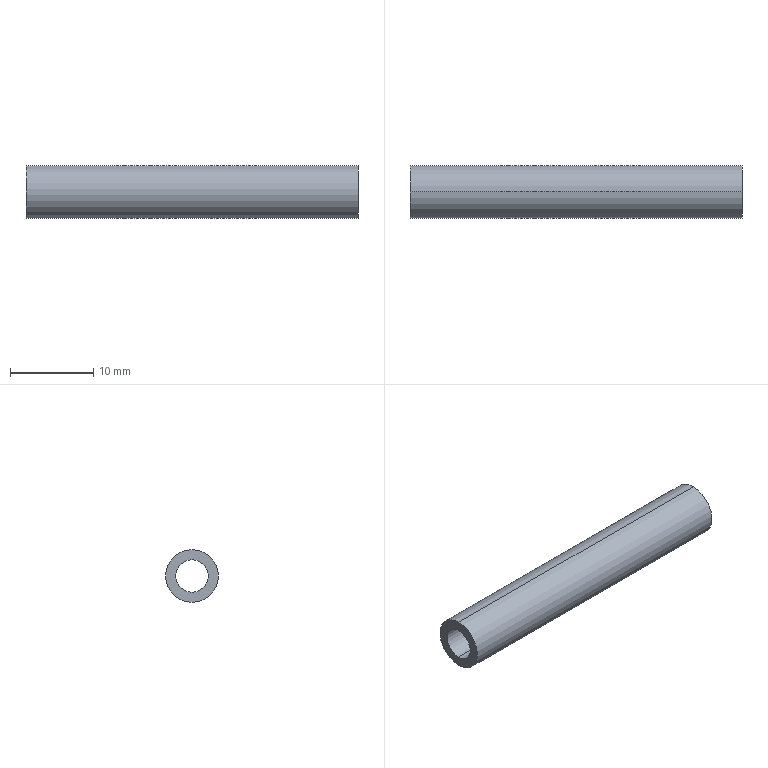Part | NX | features BREP 1 | 1 solid | 6 faces | box 40 x 6.35 x 6.35 mm | volume 786.479 mm3 | cylinder 4 | plane 2 | commonest cylinder face diameters 3.91 x2 6.35 x2
STEP:
#1=CARTESIAN_POINT('',(-107.,-470.557,3.175));
#2=VERTEX_POINT('',#1);
#3=CARTESIAN_POINT('',(-107.,-470.557,-3.175));
#4=VERTEX_POINT('',#3);
#5=CARTESIAN_POINT('',(-107.,-470.557,0.));
#6=DIRECTION('',(-1.,0.,0.));
#7=DIRECTION('',(0.,0.,1.));
#8=AXIS2_PLACEMENT_3D('',#5,#6,#7);
#9=CIRCLE('',#8,3.175);
#10=EDGE_CURVE('',#2,#4,#9,.T.);
#11=ORIENTED_EDGE('',*,*,#10,.T.);
#12=CARTESIAN_POINT('',(-107.,-470.557,0.));
#13=DIRECTION('',(-1.,0.,0.));
#14=DIRECTION('',(0.,0.,-1.));
#15=AXIS2_PLACEMENT_3D('',#12,#13,#14);
#16=CIRCLE('',#15,3.175);
#17=EDGE_CURVE('',#4,#2,#16,.T.);
#18=ORIENTED_EDGE('',*,*,#17,.T.);
#19=EDGE_LOOP('',(#11,#18));
#20=FACE_BOUND('',#19,.T.);
#21=CARTESIAN_POINT('',(-107.,-470.557,-1.955));
#22=VERTEX_POINT('',#21);
#23=CARTESIAN_POINT('',(-107.,-470.557,1.955));
#24=VERTEX_POINT('',#23);
#25=CARTESIAN_POINT('',(-107.,-470.557,0.));
#26=DIRECTION('',(1.,0.,0.));
#27=DIRECTION('',(0.,0.,-1.));
#28=AXIS2_PLACEMENT_3D('',#25,#26,#27);
#29=CIRCLE('',#28,1.955);
#30=EDGE_CURVE('',#22,#24,#29,.T.);
#31=ORIENTED_EDGE('',*,*,#30,.T.);
#32=CARTESIAN_POINT('',(-107.,-470.557,0.));
#33=DIRECTION('',(1.,0.,0.));
#34=DIRECTION('',(0.,0.,1.));
#35=AXIS2_PLACEMENT_3D('',#32,#33,#34);
#36=CIRCLE('',#35,1.955);
#37=EDGE_CURVE('',#24,#22,#36,.T.);
#38=ORIENTED_EDGE('',*,*,#37,.T.);
#39=EDGE_LOOP('',(#31,#38));
#40=FACE_BOUND('',#39,.T.);
#41=CARTESIAN_POINT('',(-107.,-470.557,0.));
#42=DIRECTION('',(-1.,0.,0.));
#43=DIRECTION('',(0.,0.,1.));
#44=AXIS2_PLACEMENT_3D('',#41,#42,#43);
#45=PLANE('',#44);
#46=ADVANCED_FACE('',(#20,#40),#45,.T.);
#47=ORIENTED_EDGE('',*,*,#17,.F.);
#48=CARTESIAN_POINT('',(-67.,-470.557,-3.175));
#49=VERTEX_POINT('',#48);
#50=CARTESIAN_POINT('',(-67.,-470.557,-3.175));
#51=DIRECTION('',(-1.,0.,0.));
#52=VECTOR('',#51,1000.);
#53=LINE('',#50,#52);
#54=EDGE_CURVE('',#49,#4,#53,.T.);
#55=ORIENTED_EDGE('',*,*,#54,.F.);
#56=CARTESIAN_POINT('',(-67.,-470.557,3.175));
#57=VERTEX_POINT('',#56);
#58=CARTESIAN_POINT('',(-67.,-470.557,0.));
#59=DIRECTION('',(1.,0.,0.));
#60=DIRECTION('',(0.,0.,1.));
#61=AXIS2_PLACEMENT_3D('',#58,#59,#60);
#62=CIRCLE('',#61,3.175);
#63=EDGE_CURVE('',#57,#49,#62,.T.);
#64=ORIENTED_EDGE('',*,*,#63,.F.);
#65=CARTESIAN_POINT('',(-67.,-470.557,3.175));
#66=DIRECTION('',(-1.,0.,0.));
#67=VECTOR('',#66,1000.);
#68=LINE('',#65,#67);
#69=EDGE_CURVE('',#57,#2,#68,.T.);
#70=ORIENTED_EDGE('',*,*,#69,.T.);
#71=EDGE_LOOP('',(#47,#55,#64,#70));
#72=FACE_BOUND('',#71,.T.);
#73=CARTESIAN_POINT('',(-107.,-470.557,0.));
#74=DIRECTION('',(1.,0.,0.));
#75=DIRECTION('',(0.,0.,-1.));
#76=AXIS2_PLACEMENT_3D('',#73,#74,#75);
#77=CYLINDRICAL_SURFACE('',#76,3.175);
#78=ADVANCED_FACE('',(#72),#77,.T.);
#79=ORIENTED_EDGE('',*,*,#69,.F.);
#80=CARTESIAN_POINT('',(-67.,-470.557,0.));
#81=DIRECTION('',(1.,0.,0.));
#82=DIRECTION('',(0.,0.,-1.));
#83=AXIS2_PLACEMENT_3D('',#80,#81,#82);
#84=CIRCLE('',#83,3.175);
#85=EDGE_CURVE('',#49,#57,#84,.T.);
#86=ORIENTED_EDGE('',*,*,#85,.F.);
#87=ORIENTED_EDGE('',*,*,#54,.T.);
#88=ORIENTED_EDGE('',*,*,#10,.F.);
#89=EDGE_LOOP('',(#79,#86,#87,#88));
#90=FACE_BOUND('',#89,.T.);
#91=CARTESIAN_POINT('',(-107.,-470.557,0.));
#92=DIRECTION('',(1.,0.,0.));
#93=DIRECTION('',(0.,0.,-1.));
#94=AXIS2_PLACEMENT_3D('',#91,#92,#93);
#95=CYLINDRICAL_SURFACE('',#94,3.175);
#96=ADVANCED_FACE('',(#90),#95,.T.);
#97=ORIENTED_EDGE('',*,*,#85,.T.);
#98=ORIENTED_EDGE('',*,*,#63,.T.);
#99=EDGE_LOOP('',(#97,#98));
#100=FACE_BOUND('',#99,.T.);
#101=CARTESIAN_POINT('',(-67.,-470.557,1.955));
#102=VERTEX_POINT('',#101);
#103=CARTESIAN_POINT('',(-67.,-470.557,-1.955));
#104=VERTEX_POINT('',#103);
#105=CARTESIAN_POINT('',(-67.,-470.557,0.));
#106=DIRECTION('',(-1.,0.,0.));
#107=DIRECTION('',(0.,0.,1.));
#108=AXIS2_PLACEMENT_3D('',#105,#106,#107);
#109=CIRCLE('',#108,1.955);
#110=EDGE_CURVE('',#102,#104,#109,.T.);
#111=ORIENTED_EDGE('',*,*,#110,.T.);
#112=CARTESIAN_POINT('',(-67.,-470.557,0.));
#113=DIRECTION('',(-1.,0.,0.));
#114=DIRECTION('',(0.,0.,-1.));
#115=AXIS2_PLACEMENT_3D('',#112,#113,#114);
#116=CIRCLE('',#115,1.955);
#117=EDGE_CURVE('',#104,#102,#116,.T.);
#118=ORIENTED_EDGE('',*,*,#117,.T.);
#119=EDGE_LOOP('',(#111,#118));
#120=FACE_BOUND('',#119,.T.);
#121=CARTESIAN_POINT('',(-67.,-470.557,0.));
#122=DIRECTION('',(-1.,0.,0.));
#123=DIRECTION('',(0.,0.,1.));
#124=AXIS2_PLACEMENT_3D('',#121,#122,#123);
#125=PLANE('',#124);
#126=ADVANCED_FACE('',(#100,#120),#125,.F.);
#127=CARTESIAN_POINT('',(-67.,-470.557,1.955));
#128=DIRECTION('',(-1.,0.,0.));
#129=VECTOR('',#128,1000.);
#130=LINE('',#127,#129);
#131=EDGE_CURVE('',#24,#102,#130,.F.);
#132=ORIENTED_EDGE('',*,*,#131,.T.);
#133=ORIENTED_EDGE('',*,*,#117,.F.);
#134=CARTESIAN_POINT('',(-67.,-470.557,-1.955));
#135=DIRECTION('',(-1.,0.,0.));
#136=VECTOR('',#135,1000.);
#137=LINE('',#134,#136);
#138=EDGE_CURVE('',#22,#104,#137,.F.);
#139=ORIENTED_EDGE('',*,*,#138,.F.);
#140=ORIENTED_EDGE('',*,*,#37,.F.);
#141=EDGE_LOOP('',(#132,#133,#139,#140));
#142=FACE_BOUND('',#141,.T.);
#143=CARTESIAN_POINT('',(-107.,-470.557,0.));
#144=DIRECTION('',(1.,0.,0.));
#145=DIRECTION('',(0.,0.,-1.));
#146=AXIS2_PLACEMENT_3D('',#143,#144,#145);
#147=CYLINDRICAL_SURFACE('',#146,1.955);
#148=ADVANCED_FACE('',(#142),#147,.F.);
#149=ORIENTED_EDGE('',*,*,#30,.F.);
#150=ORIENTED_EDGE('',*,*,#138,.T.);
#151=ORIENTED_EDGE('',*,*,#110,.F.);
#152=ORIENTED_EDGE('',*,*,#131,.F.);
#153=EDGE_LOOP('',(#149,#150,#151,#152));
#154=FACE_BOUND('',#153,.T.);
#155=CARTESIAN_POINT('',(-107.,-470.557,0.));
#156=DIRECTION('',(1.,0.,0.));
#157=DIRECTION('',(0.,0.,-1.));
#158=AXIS2_PLACEMENT_3D('',#155,#156,#157);
#159=CYLINDRICAL_SURFACE('',#158,1.955);
#160=ADVANCED_FACE('',(#154),#159,.F.);
#161=CLOSED_SHELL('',(#46,#78,#96,#126,#148,#160));
#162=MANIFOLD_SOLID_BREP('',#161);
#163=(LENGTH_UNIT()NAMED_UNIT(*)SI_UNIT(.MILLI.,.METRE.));
#164=UNCERTAINTY_MEASURE_WITH_UNIT(LENGTH_MEASURE(0.00001),#163,'','');
#165=(NAMED_UNIT(*)PLANE_ANGLE_UNIT()SI_UNIT($,.RADIAN.));
#166=(NAMED_UNIT(*)SI_UNIT($,.STERADIAN.)SOLID_ANGLE_UNIT());
#167=(GEOMETRIC_REPRESENTATION_CONTEXT(3)GLOBAL_UNCERTAINTY_ASSIGNED_CONTEXT((#164))GLOBAL_UNIT_ASSIGNED_CONTEXT((#163,#165,#166))REPRESENTATION_CONTEXT('',''));
#168=ADVANCED_BREP_SHAPE_REPRESENTATION('',(#162),#167);